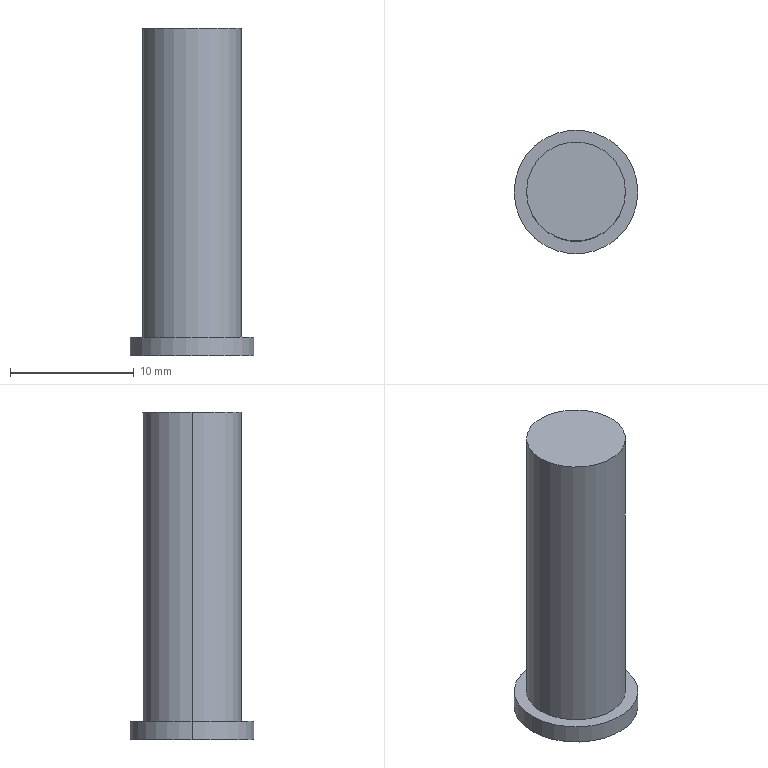Part | SolidWorks | features Extrusion 1, ICE 1 | 1 solid | 7 faces | box 10 x 10 x 26.5 mm | volume 1374 mm3 | cylinder 4 | plane 3 | commonest cylinder face diameters 8 x2 10 x2
STEP:
#1=CARTESIAN_POINT('',(4.,0.,26.5));
#2=VERTEX_POINT('',#1);
#3=CARTESIAN_POINT('',(-4.,0.,26.5));
#4=VERTEX_POINT('',#3);
#5=CARTESIAN_POINT('',(0.,0.,26.5));
#6=DIRECTION('',(0.,0.,1.));
#7=DIRECTION('',(1.,0.,0.));
#8=AXIS2_PLACEMENT_3D('',#5,#6,#7);
#9=CIRCLE('',#8,4.);
#10=EDGE_CURVE('',#2,#4,#9,.T.);
#11=ORIENTED_EDGE('',*,*,#10,.F.);
#12=CARTESIAN_POINT('',(4.,0.,1.5));
#13=VERTEX_POINT('',#12);
#14=CARTESIAN_POINT('',(4.,0.,26.5));
#15=DIRECTION('',(0.,0.,-1.));
#16=VECTOR('',#15,1000.);
#17=LINE('',#14,#16);
#18=EDGE_CURVE('',#2,#13,#17,.T.);
#19=ORIENTED_EDGE('',*,*,#18,.T.);
#20=CARTESIAN_POINT('',(-4.,0.,1.5));
#21=VERTEX_POINT('',#20);
#22=CARTESIAN_POINT('',(0.,0.,1.5));
#23=DIRECTION('',(0.,0.,1.));
#24=DIRECTION('',(1.,0.,0.));
#25=AXIS2_PLACEMENT_3D('',#22,#23,#24);
#26=CIRCLE('',#25,4.);
#27=EDGE_CURVE('',#13,#21,#26,.T.);
#28=ORIENTED_EDGE('',*,*,#27,.T.);
#29=CARTESIAN_POINT('',(-4.,0.,26.5));
#30=DIRECTION('',(0.,0.,-1.));
#31=VECTOR('',#30,1000.);
#32=LINE('',#29,#31);
#33=EDGE_CURVE('',#4,#21,#32,.T.);
#34=ORIENTED_EDGE('',*,*,#33,.F.);
#35=EDGE_LOOP('',(#11,#19,#28,#34));
#36=FACE_OUTER_BOUND('',#35,.T.);
#37=CARTESIAN_POINT('',(0.,0.,26.5));
#38=DIRECTION('',(0.,0.,-1.));
#39=DIRECTION('',(-1.,0.,0.));
#40=AXIS2_PLACEMENT_3D('',#37,#38,#39);
#41=CYLINDRICAL_SURFACE('',#40,4.);
#42=ADVANCED_FACE('',(#36),#41,.T.);
#43=CARTESIAN_POINT('',(5.,0.,1.5));
#44=VERTEX_POINT('',#43);
#45=CARTESIAN_POINT('',(-5.,0.,1.5));
#46=VERTEX_POINT('',#45);
#47=CARTESIAN_POINT('',(0.,0.,1.5));
#48=DIRECTION('',(0.,0.,1.));
#49=DIRECTION('',(1.,0.,0.));
#50=AXIS2_PLACEMENT_3D('',#47,#48,#49);
#51=CIRCLE('',#50,5.);
#52=EDGE_CURVE('',#44,#46,#51,.T.);
#53=ORIENTED_EDGE('',*,*,#52,.F.);
#54=CARTESIAN_POINT('',(5.,0.,0.));
#55=VERTEX_POINT('',#54);
#56=CARTESIAN_POINT('',(5.,0.,1.5));
#57=DIRECTION('',(0.,0.,-1.));
#58=VECTOR('',#57,1000.);
#59=LINE('',#56,#58);
#60=EDGE_CURVE('',#44,#55,#59,.T.);
#61=ORIENTED_EDGE('',*,*,#60,.T.);
#62=CARTESIAN_POINT('',(-5.,0.,0.));
#63=VERTEX_POINT('',#62);
#64=CARTESIAN_POINT('',(0.,0.,0.));
#65=DIRECTION('',(0.,0.,1.));
#66=DIRECTION('',(1.,0.,0.));
#67=AXIS2_PLACEMENT_3D('',#64,#65,#66);
#68=CIRCLE('',#67,5.);
#69=EDGE_CURVE('',#55,#63,#68,.T.);
#70=ORIENTED_EDGE('',*,*,#69,.T.);
#71=CARTESIAN_POINT('',(-5.,0.,1.5));
#72=DIRECTION('',(0.,0.,-1.));
#73=VECTOR('',#72,1000.);
#74=LINE('',#71,#73);
#75=EDGE_CURVE('',#46,#63,#74,.T.);
#76=ORIENTED_EDGE('',*,*,#75,.F.);
#77=EDGE_LOOP('',(#53,#61,#70,#76));
#78=FACE_OUTER_BOUND('',#77,.T.);
#79=CARTESIAN_POINT('',(0.,0.,1.5));
#80=DIRECTION('',(0.,0.,-1.));
#81=DIRECTION('',(-1.,0.,0.));
#82=AXIS2_PLACEMENT_3D('',#79,#80,#81);
#83=CYLINDRICAL_SURFACE('',#82,5.);
#84=ADVANCED_FACE('',(#78),#83,.T.);
#85=ORIENTED_EDGE('',*,*,#60,.F.);
#86=CARTESIAN_POINT('',(0.,0.,1.5));
#87=DIRECTION('',(0.,0.,1.));
#88=DIRECTION('',(1.,0.,0.));
#89=AXIS2_PLACEMENT_3D('',#86,#87,#88);
#90=CIRCLE('',#89,5.);
#91=EDGE_CURVE('',#46,#44,#90,.T.);
#92=ORIENTED_EDGE('',*,*,#91,.F.);
#93=ORIENTED_EDGE('',*,*,#75,.T.);
#94=CARTESIAN_POINT('',(0.,0.,0.));
#95=DIRECTION('',(0.,0.,1.));
#96=DIRECTION('',(1.,0.,0.));
#97=AXIS2_PLACEMENT_3D('',#94,#95,#96);
#98=CIRCLE('',#97,5.);
#99=EDGE_CURVE('',#63,#55,#98,.T.);
#100=ORIENTED_EDGE('',*,*,#99,.T.);
#101=EDGE_LOOP('',(#85,#92,#93,#100));
#102=FACE_OUTER_BOUND('',#101,.T.);
#103=CARTESIAN_POINT('',(0.,0.,1.5));
#104=DIRECTION('',(0.,0.,-1.));
#105=DIRECTION('',(-1.,0.,0.));
#106=AXIS2_PLACEMENT_3D('',#103,#104,#105);
#107=CYLINDRICAL_SURFACE('',#106,5.);
#108=ADVANCED_FACE('',(#102),#107,.T.);
#109=CARTESIAN_POINT('',(0.,0.,1.5));
#110=DIRECTION('',(0.,0.,1.));
#111=DIRECTION('',(1.,0.,0.));
#112=AXIS2_PLACEMENT_3D('',#109,#110,#111);
#113=CIRCLE('',#112,4.);
#114=EDGE_CURVE('',#21,#13,#113,.T.);
#115=ORIENTED_EDGE('',*,*,#114,.F.);
#116=ORIENTED_EDGE('',*,*,#27,.F.);
#117=EDGE_LOOP('',(#115,#116));
#118=FACE_BOUND('',#117,.T.);
#119=ORIENTED_EDGE('',*,*,#91,.T.);
#120=ORIENTED_EDGE('',*,*,#52,.T.);
#121=EDGE_LOOP('',(#119,#120));
#122=FACE_OUTER_BOUND('',#121,.T.);
#123=CARTESIAN_POINT('',(0.,0.,1.5));
#124=DIRECTION('',(0.,0.,1.));
#125=DIRECTION('',(1.,0.,0.));
#126=AXIS2_PLACEMENT_3D('',#123,#124,#125);
#127=PLANE('',#126);
#128=ADVANCED_FACE('',(#118,#122),#127,.T.);
#129=ORIENTED_EDGE('',*,*,#99,.F.);
#130=ORIENTED_EDGE('',*,*,#69,.F.);
#131=EDGE_LOOP('',(#129,#130));
#132=FACE_OUTER_BOUND('',#131,.T.);
#133=CARTESIAN_POINT('',(0.,0.,0.));
#134=DIRECTION('',(0.,0.,1.));
#135=DIRECTION('',(1.,0.,0.));
#136=AXIS2_PLACEMENT_3D('',#133,#134,#135);
#137=PLANE('',#136);
#138=ADVANCED_FACE('',(#132),#137,.F.);
#139=ORIENTED_EDGE('',*,*,#18,.F.);
#140=CARTESIAN_POINT('',(0.,0.,26.5));
#141=DIRECTION('',(0.,0.,1.));
#142=DIRECTION('',(1.,0.,0.));
#143=AXIS2_PLACEMENT_3D('',#140,#141,#142);
#144=CIRCLE('',#143,4.);
#145=EDGE_CURVE('',#4,#2,#144,.T.);
#146=ORIENTED_EDGE('',*,*,#145,.F.);
#147=ORIENTED_EDGE('',*,*,#33,.T.);
#148=ORIENTED_EDGE('',*,*,#114,.T.);
#149=EDGE_LOOP('',(#139,#146,#147,#148));
#150=FACE_OUTER_BOUND('',#149,.T.);
#151=CARTESIAN_POINT('',(0.,0.,26.5));
#152=DIRECTION('',(0.,0.,-1.));
#153=DIRECTION('',(-1.,0.,0.));
#154=AXIS2_PLACEMENT_3D('',#151,#152,#153);
#155=CYLINDRICAL_SURFACE('',#154,4.);
#156=ADVANCED_FACE('',(#150),#155,.T.);
#157=ORIENTED_EDGE('',*,*,#145,.T.);
#158=ORIENTED_EDGE('',*,*,#10,.T.);
#159=EDGE_LOOP('',(#157,#158));
#160=FACE_OUTER_BOUND('',#159,.T.);
#161=CARTESIAN_POINT('',(0.,0.,26.5));
#162=DIRECTION('',(0.,0.,1.));
#163=DIRECTION('',(1.,0.,0.));
#164=AXIS2_PLACEMENT_3D('',#161,#162,#163);
#165=PLANE('',#164);
#166=ADVANCED_FACE('',(#160),#165,.T.);
#167=CLOSED_SHELL('',(#42,#84,#108,#128,#138,#156,#166));
#168=MANIFOLD_SOLID_BREP('',#167);
#169=CARTESIAN_POINT('',(0.,0.,0.));
#170=DIRECTION('',(0.,0.,1.));
#171=DIRECTION('',(1.,0.,0.));
#172=AXIS2_PLACEMENT_3D('',#169,#170,#171);
#173=(LENGTH_UNIT()NAMED_UNIT(*)SI_UNIT(.MILLI.,.METRE.));
#174=UNCERTAINTY_MEASURE_WITH_UNIT(LENGTH_MEASURE(0.00001),#173,'','');
#175=(NAMED_UNIT(*)PLANE_ANGLE_UNIT()SI_UNIT($,.RADIAN.));
#176=(NAMED_UNIT(*)SI_UNIT($,.STERADIAN.)SOLID_ANGLE_UNIT());
#177=(GEOMETRIC_REPRESENTATION_CONTEXT(3)GLOBAL_UNCERTAINTY_ASSIGNED_CONTEXT((#174))GLOBAL_UNIT_ASSIGNED_CONTEXT((#173,#175,#176))REPRESENTATION_CONTEXT('',''));
#178=ADVANCED_BREP_SHAPE_REPRESENTATION('',(#168,#172),#177);